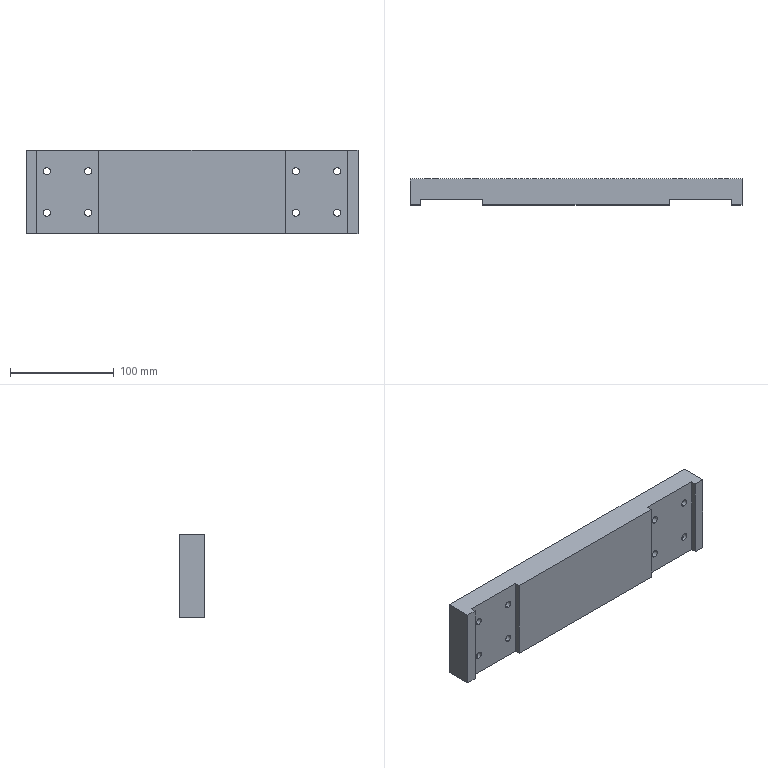Part | SolidWorks | features BaseBody 1 | 1 solid | 70 faces | box 320 x 25 x 80 mm | volume 576438 mm3 | cylinder 42 | plane 22 | cone 6 | commonest cylinder face diameters 7 x16 13 x16 5 x10